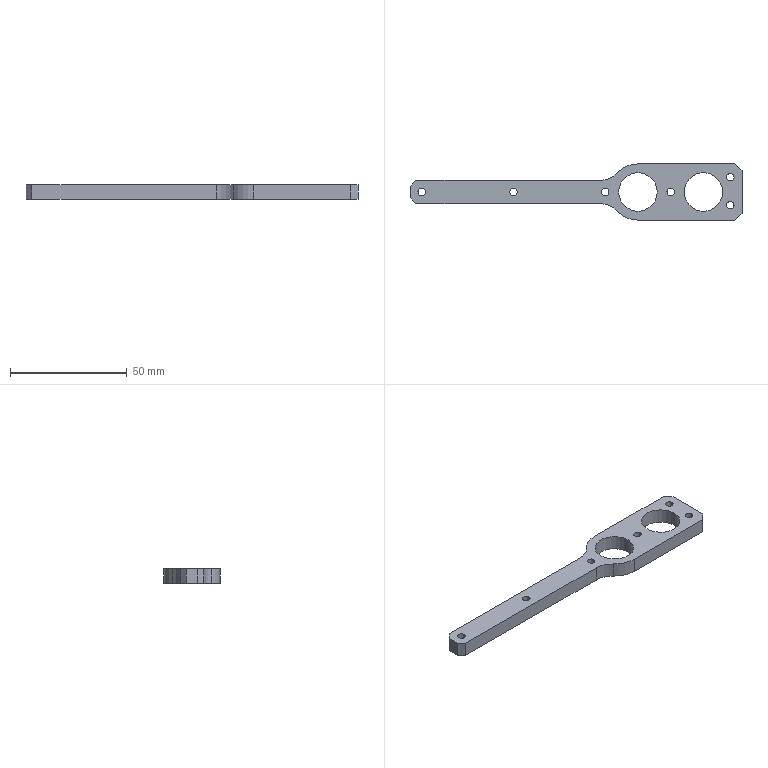Part | SolidWorks | features BaseBody 1 | 1 solid | 32 faces | box 142 x 24 x 6.35 mm | volume 10590 mm3 | cylinder 20 | plane 12 | commonest cylinder face diameters 3.2 x12 16.51 x4 20 x2 24 x2
STEP:
#1=CARTESIAN_POINT('',(-37.329,0.,6.35));
#2=VERTEX_POINT('',#1);
#3=CARTESIAN_POINT('',(-34.129,0.,6.35));
#4=VERTEX_POINT('',#3);
#5=CARTESIAN_POINT('',(-35.729,0.,6.35));
#6=DIRECTION('',(0.,0.,1.));
#7=DIRECTION('',(-1.,0.,0.));
#8=AXIS2_PLACEMENT_3D('',#5,#6,#7);
#9=CIRCLE('',#8,1.6);
#10=EDGE_CURVE('',#2,#4,#9,.T.);
#11=ORIENTED_EDGE('',*,*,#10,.T.);
#12=CARTESIAN_POINT('',(-34.129,0.,0.));
#13=VERTEX_POINT('',#12);
#14=CARTESIAN_POINT('',(-34.129,0.,6.35));
#15=DIRECTION('',(0.,0.,-1.));
#16=VECTOR('',#15,1000.);
#17=LINE('',#14,#16);
#18=EDGE_CURVE('',#4,#13,#17,.T.);
#19=ORIENTED_EDGE('',*,*,#18,.T.);
#20=CARTESIAN_POINT('',(-37.329,0.,0.));
#21=VERTEX_POINT('',#20);
#22=CARTESIAN_POINT('',(-35.729,0.,0.));
#23=DIRECTION('',(0.,0.,-1.));
#24=DIRECTION('',(-1.,0.,0.));
#25=AXIS2_PLACEMENT_3D('',#22,#23,#24);
#26=CIRCLE('',#25,1.6);
#27=EDGE_CURVE('',#13,#21,#26,.T.);
#28=ORIENTED_EDGE('',*,*,#27,.T.);
#29=CARTESIAN_POINT('',(-37.329,0.,6.35));
#30=DIRECTION('',(0.,0.,-1.));
#31=VECTOR('',#30,1000.);
#32=LINE('',#29,#31);
#33=EDGE_CURVE('',#2,#21,#32,.T.);
#34=ORIENTED_EDGE('',*,*,#33,.F.);
#35=EDGE_LOOP('',(#11,#19,#28,#34));
#36=FACE_OUTER_BOUND('',#35,.T.);
#37=CARTESIAN_POINT('',(-35.729,0.,6.35));
#38=DIRECTION('',(0.,0.,-1.));
#39=DIRECTION('',(-1.,0.,0.));
#40=AXIS2_PLACEMENT_3D('',#37,#38,#39);
#41=CYLINDRICAL_SURFACE('',#40,1.6);
#42=ADVANCED_FACE('',(#36),#41,.F.);
#43=CARTESIAN_POINT('',(58.621,-5.603,6.35));
#44=VERTEX_POINT('',#43);
#45=CARTESIAN_POINT('',(55.421,-5.603,6.35));
#46=VERTEX_POINT('',#45);
#47=CARTESIAN_POINT('',(57.021,-5.603,6.35));
#48=DIRECTION('',(0.,0.,-1.));
#49=DIRECTION('',(-1.,0.,0.));
#50=AXIS2_PLACEMENT_3D('',#47,#48,#49);
#51=CIRCLE('',#50,1.6);
#52=EDGE_CURVE('',#44,#46,#51,.T.);
#53=ORIENTED_EDGE('',*,*,#52,.F.);
#54=CARTESIAN_POINT('',(58.621,-5.603,0.));
#55=VERTEX_POINT('',#54);
#56=CARTESIAN_POINT('',(58.621,-5.603,6.35));
#57=DIRECTION('',(0.,0.,-1.));
#58=VECTOR('',#57,1000.);
#59=LINE('',#56,#58);
#60=EDGE_CURVE('',#44,#55,#59,.T.);
#61=ORIENTED_EDGE('',*,*,#60,.T.);
#62=CARTESIAN_POINT('',(55.421,-5.603,0.));
#63=VERTEX_POINT('',#62);
#64=CARTESIAN_POINT('',(57.021,-5.603,0.));
#65=DIRECTION('',(0.,0.,-1.));
#66=DIRECTION('',(-1.,0.,0.));
#67=AXIS2_PLACEMENT_3D('',#64,#65,#66);
#68=CIRCLE('',#67,1.6);
#69=EDGE_CURVE('',#55,#63,#68,.T.);
#70=ORIENTED_EDGE('',*,*,#69,.T.);
#71=CARTESIAN_POINT('',(55.421,-5.603,6.35));
#72=DIRECTION('',(0.,0.,-1.));
#73=VECTOR('',#72,1000.);
#74=LINE('',#71,#73);
#75=EDGE_CURVE('',#46,#63,#74,.T.);
#76=ORIENTED_EDGE('',*,*,#75,.F.);
#77=EDGE_LOOP('',(#53,#61,#70,#76));
#78=FACE_OUTER_BOUND('',#77,.T.);
#79=CARTESIAN_POINT('',(57.021,-5.603,6.35));
#80=DIRECTION('',(0.,0.,-1.));
#81=DIRECTION('',(-1.,0.,0.));
#82=AXIS2_PLACEMENT_3D('',#79,#80,#81);
#83=CYLINDRICAL_SURFACE('',#82,1.6);
#84=ADVANCED_FACE('',(#78),#83,.F.);
#85=CARTESIAN_POINT('',(-73.379,0.,6.35));
#86=VERTEX_POINT('',#85);
#87=CARTESIAN_POINT('',(-76.579,0.,6.35));
#88=VERTEX_POINT('',#87);
#89=CARTESIAN_POINT('',(-74.979,0.,6.35));
#90=DIRECTION('',(0.,0.,-1.));
#91=DIRECTION('',(-1.,0.,0.));
#92=AXIS2_PLACEMENT_3D('',#89,#90,#91);
#93=CIRCLE('',#92,1.6);
#94=EDGE_CURVE('',#86,#88,#93,.T.);
#95=ORIENTED_EDGE('',*,*,#94,.F.);
#96=CARTESIAN_POINT('',(-73.379,0.,0.));
#97=VERTEX_POINT('',#96);
#98=CARTESIAN_POINT('',(-73.379,0.,6.35));
#99=DIRECTION('',(0.,0.,-1.));
#100=VECTOR('',#99,1000.);
#101=LINE('',#98,#100);
#102=EDGE_CURVE('',#86,#97,#101,.T.);
#103=ORIENTED_EDGE('',*,*,#102,.T.);
#104=CARTESIAN_POINT('',(-76.579,0.,0.));
#105=VERTEX_POINT('',#104);
#106=CARTESIAN_POINT('',(-74.979,0.,0.));
#107=DIRECTION('',(0.,0.,-1.));
#108=DIRECTION('',(-1.,0.,0.));
#109=AXIS2_PLACEMENT_3D('',#106,#107,#108);
#110=CIRCLE('',#109,1.6);
#111=EDGE_CURVE('',#97,#105,#110,.T.);
#112=ORIENTED_EDGE('',*,*,#111,.T.);
#113=CARTESIAN_POINT('',(-76.579,0.,6.35));
#114=DIRECTION('',(0.,0.,-1.));
#115=VECTOR('',#114,1000.);
#116=LINE('',#113,#115);
#117=EDGE_CURVE('',#88,#105,#116,.T.);
#118=ORIENTED_EDGE('',*,*,#117,.F.);
#119=EDGE_LOOP('',(#95,#103,#112,#118));
#120=FACE_OUTER_BOUND('',#119,.T.);
#121=CARTESIAN_POINT('',(-74.979,0.,6.35));
#122=DIRECTION('',(0.,0.,-1.));
#123=DIRECTION('',(-1.,0.,0.));
#124=AXIS2_PLACEMENT_3D('',#121,#122,#123);
#125=CYLINDRICAL_SURFACE('',#124,1.6);
#126=ADVANCED_FACE('',(#120),#125,.F.);
#127=CARTESIAN_POINT('',(33.121,0.,6.35));
#128=VERTEX_POINT('',#127);
#129=CARTESIAN_POINT('',(29.921,0.,6.35));
#130=VERTEX_POINT('',#129);
#131=CARTESIAN_POINT('',(31.521,0.,6.35));
#132=DIRECTION('',(0.,0.,-1.));
#133=DIRECTION('',(-1.,0.,0.));
#134=AXIS2_PLACEMENT_3D('',#131,#132,#133);
#135=CIRCLE('',#134,1.6);
#136=EDGE_CURVE('',#128,#130,#135,.T.);
#137=ORIENTED_EDGE('',*,*,#136,.F.);
#138=CARTESIAN_POINT('',(33.121,0.,0.));
#139=VERTEX_POINT('',#138);
#140=CARTESIAN_POINT('',(33.121,0.,6.35));
#141=DIRECTION('',(0.,0.,-1.));
#142=VECTOR('',#141,1000.);
#143=LINE('',#140,#142);
#144=EDGE_CURVE('',#128,#139,#143,.T.);
#145=ORIENTED_EDGE('',*,*,#144,.T.);
#146=CARTESIAN_POINT('',(29.921,0.,0.));
#147=VERTEX_POINT('',#146);
#148=CARTESIAN_POINT('',(31.521,0.,0.));
#149=DIRECTION('',(0.,0.,-1.));
#150=DIRECTION('',(-1.,0.,0.));
#151=AXIS2_PLACEMENT_3D('',#148,#149,#150);
#152=CIRCLE('',#151,1.6);
#153=EDGE_CURVE('',#139,#147,#152,.T.);
#154=ORIENTED_EDGE('',*,*,#153,.T.);
#155=CARTESIAN_POINT('',(29.921,0.,6.35));
#156=DIRECTION('',(0.,0.,-1.));
#157=VECTOR('',#156,1000.);
#158=LINE('',#155,#157);
#159=EDGE_CURVE('',#130,#147,#158,.T.);
#160=ORIENTED_EDGE('',*,*,#159,.F.);
#161=EDGE_LOOP('',(#137,#145,#154,#160));
#162=FACE_OUTER_BOUND('',#161,.T.);
#163=CARTESIAN_POINT('',(31.521,0.,6.35));
#164=DIRECTION('',(0.,0.,-1.));
#165=DIRECTION('',(-1.,0.,0.));
#166=AXIS2_PLACEMENT_3D('',#163,#164,#165);
#167=CYLINDRICAL_SURFACE('',#166,1.6);
#168=ADVANCED_FACE('',(#162),#167,.F.);
#169=CARTESIAN_POINT('',(25.776,0.,6.35));
#170=VERTEX_POINT('',#169);
#171=CARTESIAN_POINT('',(9.266,0.,6.35));
#172=VERTEX_POINT('',#171);
#173=CARTESIAN_POINT('',(17.521,0.,6.35));
#174=DIRECTION('',(0.,0.,-1.));
#175=DIRECTION('',(-1.,0.,0.));
#176=AXIS2_PLACEMENT_3D('',#173,#174,#175);
#177=CIRCLE('',#176,8.255);
#178=EDGE_CURVE('',#170,#172,#177,.T.);
#179=ORIENTED_EDGE('',*,*,#178,.F.);
#180=CARTESIAN_POINT('',(25.776,0.,0.));
#181=VERTEX_POINT('',#180);
#182=CARTESIAN_POINT('',(25.776,0.,6.35));
#183=DIRECTION('',(0.,0.,-1.));
#184=VECTOR('',#183,1000.);
#185=LINE('',#182,#184);
#186=EDGE_CURVE('',#170,#181,#185,.T.);
#187=ORIENTED_EDGE('',*,*,#186,.T.);
#188=CARTESIAN_POINT('',(9.266,0.,0.));
#189=VERTEX_POINT('',#188);
#190=CARTESIAN_POINT('',(17.521,0.,0.));
#191=DIRECTION('',(0.,0.,-1.));
#192=DIRECTION('',(-1.,0.,0.));
#193=AXIS2_PLACEMENT_3D('',#190,#191,#192);
#194=CIRCLE('',#193,8.255);
#195=EDGE_CURVE('',#181,#189,#194,.T.);
#196=ORIENTED_EDGE('',*,*,#195,.T.);
#197=CARTESIAN_POINT('',(9.266,0.,6.35));
#198=DIRECTION('',(0.,0.,-1.));
#199=VECTOR('',#198,1000.);
#200=LINE('',#197,#199);
#201=EDGE_CURVE('',#172,#189,#200,.T.);
#202=ORIENTED_EDGE('',*,*,#201,.F.);
#203=EDGE_LOOP('',(#179,#187,#196,#202));
#204=FACE_OUTER_BOUND('',#203,.T.);
#205=CARTESIAN_POINT('',(17.521,0.,6.35));
#206=DIRECTION('',(0.,0.,-1.));
#207=DIRECTION('',(-1.,0.,0.));
#208=AXIS2_PLACEMENT_3D('',#205,#206,#207);
#209=CYLINDRICAL_SURFACE('',#208,8.255);
#210=ADVANCED_FACE('',(#204),#209,.F.);
#211=CARTESIAN_POINT('',(5.121,0.,6.35));
#212=VERTEX_POINT('',#211);
#213=CARTESIAN_POINT('',(1.921,0.,6.35));
#214=VERTEX_POINT('',#213);
#215=CARTESIAN_POINT('',(3.521,0.,6.35));
#216=DIRECTION('',(0.,0.,-1.));
#217=DIRECTION('',(-1.,0.,0.));
#218=AXIS2_PLACEMENT_3D('',#215,#216,#217);
#219=CIRCLE('',#218,1.6);
#220=EDGE_CURVE('',#212,#214,#219,.T.);
#221=ORIENTED_EDGE('',*,*,#220,.F.);
#222=CARTESIAN_POINT('',(5.121,0.,0.));
#223=VERTEX_POINT('',#222);
#224=CARTESIAN_POINT('',(5.121,0.,6.35));
#225=DIRECTION('',(0.,0.,-1.));
#226=VECTOR('',#225,1000.);
#227=LINE('',#224,#226);
#228=EDGE_CURVE('',#212,#223,#227,.T.);
#229=ORIENTED_EDGE('',*,*,#228,.T.);
#230=CARTESIAN_POINT('',(1.921,0.,0.));
#231=VERTEX_POINT('',#230);
#232=CARTESIAN_POINT('',(3.521,0.,0.));
#233=DIRECTION('',(0.,0.,-1.));
#234=DIRECTION('',(-1.,0.,0.));
#235=AXIS2_PLACEMENT_3D('',#232,#233,#234);
#236=CIRCLE('',#235,1.6);
#237=EDGE_CURVE('',#223,#231,#236,.T.);
#238=ORIENTED_EDGE('',*,*,#237,.T.);
#239=CARTESIAN_POINT('',(1.921,0.,6.35));
#240=DIRECTION('',(0.,0.,-1.));
#241=VECTOR('',#240,1000.);
#242=LINE('',#239,#241);
#243=EDGE_CURVE('',#214,#231,#242,.T.);
#244=ORIENTED_EDGE('',*,*,#243,.F.);
#245=EDGE_LOOP('',(#221,#229,#238,#244));
#246=FACE_OUTER_BOUND('',#245,.T.);
#247=CARTESIAN_POINT('',(3.521,0.,6.35));
#248=DIRECTION('',(0.,0.,-1.));
#249=DIRECTION('',(-1.,0.,0.));
#250=AXIS2_PLACEMENT_3D('',#247,#248,#249);
#251=CYLINDRICAL_SURFACE('',#250,1.6);
#252=ADVANCED_FACE('',(#246),#251,.F.);
#253=CARTESIAN_POINT('',(58.621,6.302,6.35));
#254=VERTEX_POINT('',#253);
#255=CARTESIAN_POINT('',(55.421,6.302,6.35));
#256=VERTEX_POINT('',#255);
#257=CARTESIAN_POINT('',(57.021,6.302,6.35));
#258=DIRECTION('',(0.,0.,-1.));
#259=DIRECTION('',(-1.,0.,0.));
#260=AXIS2_PLACEMENT_3D('',#257,#258,#259);
#261=CIRCLE('',#260,1.6);
#262=EDGE_CURVE('',#254,#256,#261,.T.);
#263=ORIENTED_EDGE('',*,*,#262,.F.);
#264=CARTESIAN_POINT('',(58.621,6.302,0.));
#265=VERTEX_POINT('',#264);
#266=CARTESIAN_POINT('',(58.621,6.302,6.35));
#267=DIRECTION('',(0.,0.,-1.));
#268=VECTOR('',#267,1000.);
#269=LINE('',#266,#268);
#270=EDGE_CURVE('',#254,#265,#269,.T.);
#271=ORIENTED_EDGE('',*,*,#270,.T.);
#272=CARTESIAN_POINT('',(55.421,6.302,0.));
#273=VERTEX_POINT('',#272);
#274=CARTESIAN_POINT('',(57.021,6.302,0.));
#275=DIRECTION('',(0.,0.,-1.));
#276=DIRECTION('',(-1.,0.,0.));
#277=AXIS2_PLACEMENT_3D('',#274,#275,#276);
#278=CIRCLE('',#277,1.6);
#279=EDGE_CURVE('',#265,#273,#278,.T.);
#280=ORIENTED_EDGE('',*,*,#279,.T.);
#281=CARTESIAN_POINT('',(55.421,6.302,6.35));
#282=DIRECTION('',(0.,0.,-1.));
#283=VECTOR('',#282,1000.);
#284=LINE('',#281,#283);
#285=EDGE_CURVE('',#256,#273,#284,.T.);
#286=ORIENTED_EDGE('',*,*,#285,.F.);
#287=EDGE_LOOP('',(#263,#271,#280,#286));
#288=FACE_OUTER_BOUND('',#287,.T.);
#289=CARTESIAN_POINT('',(57.021,6.302,6.35));
#290=DIRECTION('',(0.,0.,-1.));
#291=DIRECTION('',(-1.,0.,0.));
#292=AXIS2_PLACEMENT_3D('',#289,#290,#291);
#293=CYLINDRICAL_SURFACE('',#292,1.6);
#294=ADVANCED_FACE('',(#288),#293,.F.);
#295=CARTESIAN_POINT('',(53.776,0.,6.35));
#296=VERTEX_POINT('',#295);
#297=CARTESIAN_POINT('',(37.266,0.,6.35));
#298=VERTEX_POINT('',#297);
#299=CARTESIAN_POINT('',(45.521,0.,6.35));
#300=DIRECTION('',(0.,0.,-1.));
#301=DIRECTION('',(-1.,0.,0.));
#302=AXIS2_PLACEMENT_3D('',#299,#300,#301);
#303=CIRCLE('',#302,8.255);
#304=EDGE_CURVE('',#296,#298,#303,.T.);
#305=ORIENTED_EDGE('',*,*,#304,.F.);
#306=CARTESIAN_POINT('',(53.776,0.,0.));
#307=VERTEX_POINT('',#306);
#308=CARTESIAN_POINT('',(53.776,0.,6.35));
#309=DIRECTION('',(0.,0.,-1.));
#310=VECTOR('',#309,1000.);
#311=LINE('',#308,#310);
#312=EDGE_CURVE('',#296,#307,#311,.T.);
#313=ORIENTED_EDGE('',*,*,#312,.T.);
#314=CARTESIAN_POINT('',(37.266,0.,0.));
#315=VERTEX_POINT('',#314);
#316=CARTESIAN_POINT('',(45.521,0.,0.));
#317=DIRECTION('',(0.,0.,-1.));
#318=DIRECTION('',(-1.,0.,0.));
#319=AXIS2_PLACEMENT_3D('',#316,#317,#318);
#320=CIRCLE('',#319,8.255);
#321=EDGE_CURVE('',#307,#315,#320,.T.);
#322=ORIENTED_EDGE('',*,*,#321,.T.);
#323=CARTESIAN_POINT('',(37.266,0.,6.35));
#324=DIRECTION('',(0.,0.,-1.));
#325=VECTOR('',#324,1000.);
#326=LINE('',#323,#325);
#327=EDGE_CURVE('',#298,#315,#326,.T.);
#328=ORIENTED_EDGE('',*,*,#327,.F.);
#329=EDGE_LOOP('',(#305,#313,#322,#328));
#330=FACE_OUTER_BOUND('',#329,.T.);
#331=CARTESIAN_POINT('',(45.521,0.,6.35));
#332=DIRECTION('',(0.,0.,-1.));
#333=DIRECTION('',(-1.,0.,0.));
#334=AXIS2_PLACEMENT_3D('',#331,#332,#333);
#335=CYLINDRICAL_SURFACE('',#334,8.255);
#336=ADVANCED_FACE('',(#330),#335,.F.);
#337=ORIENTED_EDGE('',*,*,#18,.F.);
#338=CARTESIAN_POINT('',(-35.729,0.,6.35));
#339=DIRECTION('',(0.,0.,1.));
#340=DIRECTION('',(-1.,0.,0.));
#341=AXIS2_PLACEMENT_3D('',#338,#339,#340);
#342=CIRCLE('',#341,1.6);
#343=EDGE_CURVE('',#4,#2,#342,.T.);
#344=ORIENTED_EDGE('',*,*,#343,.T.);
#345=ORIENTED_EDGE('',*,*,#33,.T.);
#346=CARTESIAN_POINT('',(-35.729,0.,0.));
#347=DIRECTION('',(0.,0.,-1.));
#348=DIRECTION('',(-1.,0.,0.));
#349=AXIS2_PLACEMENT_3D('',#346,#347,#348);
#350=CIRCLE('',#349,1.6);
#351=EDGE_CURVE('',#21,#13,#350,.T.);
#352=ORIENTED_EDGE('',*,*,#351,.T.);
#353=EDGE_LOOP('',(#337,#344,#345,#352));
#354=FACE_OUTER_BOUND('',#353,.T.);
#355=CARTESIAN_POINT('',(-35.729,0.,6.35));
#356=DIRECTION('',(0.,0.,-1.));
#357=DIRECTION('',(-1.,0.,0.));
#358=AXIS2_PLACEMENT_3D('',#355,#356,#357);
#359=CYLINDRICAL_SURFACE('',#358,1.6);
#360=ADVANCED_FACE('',(#354),#359,.F.);
#361=ORIENTED_EDGE('',*,*,#351,.F.);
#362=ORIENTED_EDGE('',*,*,#27,.F.);
#363=EDGE_LOOP('',(#361,#362));
#364=FACE_BOUND('',#363,.T.);
#365=CARTESIAN_POINT('',(57.021,-5.603,0.));
#366=DIRECTION('',(0.,0.,-1.));
#367=DIRECTION('',(-1.,0.,0.));
#368=AXIS2_PLACEMENT_3D('',#365,#366,#367);
#369=CIRCLE('',#368,1.6);
#370=EDGE_CURVE('',#63,#55,#369,.T.);
#371=ORIENTED_EDGE('',*,*,#370,.F.);
#372=ORIENTED_EDGE('',*,*,#69,.F.);
#373=EDGE_LOOP('',(#371,#372));
#374=FACE_BOUND('',#373,.T.);
#375=CARTESIAN_POINT('',(-74.979,0.,0.));
#376=DIRECTION('',(0.,0.,-1.));
#377=DIRECTION('',(-1.,0.,0.));
#378=AXIS2_PLACEMENT_3D('',#375,#376,#377);
#379=CIRCLE('',#378,1.6);
#380=EDGE_CURVE('',#105,#97,#379,.T.);
#381=ORIENTED_EDGE('',*,*,#380,.F.);
#382=ORIENTED_EDGE('',*,*,#111,.F.);
#383=EDGE_LOOP('',(#381,#382));
#384=FACE_BOUND('',#383,.T.);
#385=CARTESIAN_POINT('',(31.521,0.,0.));
#386=DIRECTION('',(0.,0.,-1.));
#387=DIRECTION('',(-1.,0.,0.));
#388=AXIS2_PLACEMENT_3D('',#385,#386,#387);
#389=CIRCLE('',#388,1.6);
#390=EDGE_CURVE('',#147,#139,#389,.T.);
#391=ORIENTED_EDGE('',*,*,#390,.F.);
#392=ORIENTED_EDGE('',*,*,#153,.F.);
#393=EDGE_LOOP('',(#391,#392));
#394=FACE_BOUND('',#393,.T.);
#395=CARTESIAN_POINT('',(17.521,0.,0.));
#396=DIRECTION('',(0.,0.,-1.));
#397=DIRECTION('',(-1.,0.,0.));
#398=AXIS2_PLACEMENT_3D('',#395,#396,#397);
#399=CIRCLE('',#398,8.255);
#400=EDGE_CURVE('',#189,#181,#399,.T.);
#401=ORIENTED_EDGE('',*,*,#400,.F.);
#402=ORIENTED_EDGE('',*,*,#195,.F.);
#403=EDGE_LOOP('',(#401,#402));
#404=FACE_BOUND('',#403,.T.);
#405=CARTESIAN_POINT('',(3.521,0.,0.));
#406=DIRECTION('',(0.,0.,-1.));
#407=DIRECTION('',(-1.,0.,0.));
#408=AXIS2_PLACEMENT_3D('',#405,#406,#407);
#409=CIRCLE('',#408,1.6);
#410=EDGE_CURVE('',#231,#223,#409,.T.);
#411=ORIENTED_EDGE('',*,*,#410,.F.);
#412=ORIENTED_EDGE('',*,*,#237,.F.);
#413=EDGE_LOOP('',(#411,#412));
#414=FACE_BOUND('',#413,.T.);
#415=CARTESIAN_POINT('',(57.021,6.302,0.));
#416=DIRECTION('',(0.,0.,-1.));
#417=DIRECTION('',(-1.,0.,0.));
#418=AXIS2_PLACEMENT_3D('',#415,#416,#417);
#419=CIRCLE('',#418,1.6);
#420=EDGE_CURVE('',#273,#265,#419,.T.);
#421=ORIENTED_EDGE('',*,*,#420,.F.);
#422=ORIENTED_EDGE('',*,*,#279,.F.);
#423=EDGE_LOOP('',(#421,#422));
#424=FACE_BOUND('',#423,.T.);
#425=CARTESIAN_POINT('',(45.521,0.,0.));
#426=DIRECTION('',(0.,0.,-1.));
#427=DIRECTION('',(-1.,0.,0.));
#428=AXIS2_PLACEMENT_3D('',#425,#426,#427);
#429=CIRCLE('',#428,8.255);
#430=EDGE_CURVE('',#315,#307,#429,.T.);
#431=ORIENTED_EDGE('',*,*,#430,.F.);
#432=ORIENTED_EDGE('',*,*,#321,.F.);
#433=EDGE_LOOP('',(#431,#432));
#434=FACE_BOUND('',#433,.T.);
#435=CARTESIAN_POINT('',(8.742,8.182,0.));
#436=VERTEX_POINT('',#435);
#437=CARTESIAN_POINT('',(1.427,5.,0.));
#438=VERTEX_POINT('',#437);
#439=CARTESIAN_POINT('',(1.427,15.,0.));
#440=DIRECTION('',(0.,0.,-1.));
#441=DIRECTION('',(-1.,0.,0.));
#442=AXIS2_PLACEMENT_3D('',#439,#440,#441);
#443=CIRCLE('',#442,10.);
#444=EDGE_CURVE('',#436,#438,#443,.T.);
#445=ORIENTED_EDGE('',*,*,#444,.F.);
#446=CARTESIAN_POINT('',(17.521,12.,0.));
#447=VERTEX_POINT('',#446);
#448=CARTESIAN_POINT('',(17.521,0.,0.));
#449=DIRECTION('',(0.,0.,1.));
#450=DIRECTION('',(-1.,0.,0.));
#451=AXIS2_PLACEMENT_3D('',#448,#449,#450);
#452=CIRCLE('',#451,12.);
#453=EDGE_CURVE('',#447,#436,#452,.T.);
#454=ORIENTED_EDGE('',*,*,#453,.F.);
#455=CARTESIAN_POINT('',(59.021,12.,0.));
#456=VERTEX_POINT('',#455);
#457=CARTESIAN_POINT('',(-8.979,12.,0.));
#458=DIRECTION('',(-1.,0.,0.));
#459=VECTOR('',#458,1000.);
#460=LINE('',#457,#459);
#461=EDGE_CURVE('',#456,#447,#460,.T.);
#462=ORIENTED_EDGE('',*,*,#461,.F.);
#463=CARTESIAN_POINT('',(62.021,9.,0.));
#464=VERTEX_POINT('',#463);
#465=CARTESIAN_POINT('',(59.021,12.,0.));
#466=DIRECTION('',(-0.7071,0.7071,0.));
#467=VECTOR('',#466,1000.);
#468=LINE('',#465,#467);
#469=EDGE_CURVE('',#464,#456,#468,.T.);
#470=ORIENTED_EDGE('',*,*,#469,.F.);
#471=CARTESIAN_POINT('',(62.021,-9.,0.));
#472=VERTEX_POINT('',#471);
#473=CARTESIAN_POINT('',(62.021,0.,0.));
#474=DIRECTION('',(0.,1.,0.));
#475=VECTOR('',#474,1000.);
#476=LINE('',#473,#475);
#477=EDGE_CURVE('',#472,#464,#476,.T.);
#478=ORIENTED_EDGE('',*,*,#477,.F.);
#479=CARTESIAN_POINT('',(59.021,-12.,0.));
#480=VERTEX_POINT('',#479);
#481=CARTESIAN_POINT('',(62.021,-9.,0.));
#482=DIRECTION('',(0.7071,0.7071,0.));
#483=VECTOR('',#482,1000.);
#484=LINE('',#481,#483);
#485=EDGE_CURVE('',#480,#472,#484,.T.);
#486=ORIENTED_EDGE('',*,*,#485,.F.);
#487=CARTESIAN_POINT('',(17.521,-12.,0.));
#488=VERTEX_POINT('',#487);
#489=CARTESIAN_POINT('',(-8.979,-12.,0.));
#490=DIRECTION('',(1.,0.,0.));
#491=VECTOR('',#490,1000.);
#492=LINE('',#489,#491);
#493=EDGE_CURVE('',#488,#480,#492,.T.);
#494=ORIENTED_EDGE('',*,*,#493,.F.);
#495=CARTESIAN_POINT('',(8.742,-8.182,0.));
#496=VERTEX_POINT('',#495);
#497=CARTESIAN_POINT('',(17.521,0.,0.));
#498=DIRECTION('',(0.,0.,1.));
#499=DIRECTION('',(-1.,0.,0.));
#500=AXIS2_PLACEMENT_3D('',#497,#498,#499);
#501=CIRCLE('',#500,12.);
#502=EDGE_CURVE('',#496,#488,#501,.T.);
#503=ORIENTED_EDGE('',*,*,#502,.F.);
#504=CARTESIAN_POINT('',(1.427,-5.,0.));
#505=VERTEX_POINT('',#504);
#506=CARTESIAN_POINT('',(1.427,-15.,0.));
#507=DIRECTION('',(0.,0.,-1.));
#508=DIRECTION('',(-1.,0.,0.));
#509=AXIS2_PLACEMENT_3D('',#506,#507,#508);
#510=CIRCLE('',#509,10.);
#511=EDGE_CURVE('',#505,#496,#510,.T.);
#512=ORIENTED_EDGE('',*,*,#511,.F.);
#513=CARTESIAN_POINT('',(-77.439,-5.,0.));
#514=VERTEX_POINT('',#513);
#515=CARTESIAN_POINT('',(-8.979,-5.,0.));
#516=DIRECTION('',(1.,0.,0.));
#517=VECTOR('',#516,1000.);
#518=LINE('',#515,#517);
#519=EDGE_CURVE('',#514,#505,#518,.T.);
#520=ORIENTED_EDGE('',*,*,#519,.F.);
#521=CARTESIAN_POINT('',(-79.979,-2.46,0.));
#522=VERTEX_POINT('',#521);
#523=CARTESIAN_POINT('',(-77.439,-5.,0.));
#524=DIRECTION('',(0.7071,-0.7071,0.));
#525=VECTOR('',#524,1000.);
#526=LINE('',#523,#525);
#527=EDGE_CURVE('',#522,#514,#526,.T.);
#528=ORIENTED_EDGE('',*,*,#527,.F.);
#529=CARTESIAN_POINT('',(-79.979,2.46,0.));
#530=VERTEX_POINT('',#529);
#531=CARTESIAN_POINT('',(-79.979,0.,0.));
#532=DIRECTION('',(0.,-1.,0.));
#533=VECTOR('',#532,1000.);
#534=LINE('',#531,#533);
#535=EDGE_CURVE('',#530,#522,#534,.T.);
#536=ORIENTED_EDGE('',*,*,#535,.F.);
#537=CARTESIAN_POINT('',(-77.439,5.,0.));
#538=VERTEX_POINT('',#537);
#539=CARTESIAN_POINT('',(-79.979,2.46,0.));
#540=DIRECTION('',(-0.7071,-0.7071,0.));
#541=VECTOR('',#540,1000.);
#542=LINE('',#539,#541);
#543=EDGE_CURVE('',#538,#530,#542,.T.);
#544=ORIENTED_EDGE('',*,*,#543,.F.);
#545=CARTESIAN_POINT('',(-8.979,5.,0.));
#546=DIRECTION('',(-1.,0.,0.));
#547=VECTOR('',#546,1000.);
#548=LINE('',#545,#547);
#549=EDGE_CURVE('',#438,#538,#548,.T.);
#550=ORIENTED_EDGE('',*,*,#549,.F.);
#551=EDGE_LOOP('',(#445,#454,#462,#470,#478,#486,#494,#503,#512,#520,#528,#536,#544,#550));
#552=FACE_OUTER_BOUND('',#551,.T.);
#553=CARTESIAN_POINT('',(-79.979,-12.,0.));
#554=DIRECTION('',(0.,0.,1.));
#555=DIRECTION('',(1.,0.,0.));
#556=AXIS2_PLACEMENT_3D('',#553,#554,#555);
#557=PLANE('',#556);
#558=ADVANCED_FACE('',(#364,#374,#384,#394,#404,#414,#424,#434,#552),#557,.F.);
#559=ORIENTED_EDGE('',*,*,#10,.F.);
#560=ORIENTED_EDGE('',*,*,#343,.F.);
#561=EDGE_LOOP('',(#559,#560));
#562=FACE_BOUND('',#561,.T.);
#563=CARTESIAN_POINT('',(57.021,-5.603,6.35));
#564=DIRECTION('',(0.,0.,-1.));
#565=DIRECTION('',(-1.,0.,0.));
#566=AXIS2_PLACEMENT_3D('',#563,#564,#565);
#567=CIRCLE('',#566,1.6);
#568=EDGE_CURVE('',#46,#44,#567,.T.);
#569=ORIENTED_EDGE('',*,*,#568,.T.);
#570=ORIENTED_EDGE('',*,*,#52,.T.);
#571=EDGE_LOOP('',(#569,#570));
#572=FACE_BOUND('',#571,.T.);
#573=CARTESIAN_POINT('',(-74.979,0.,6.35));
#574=DIRECTION('',(0.,0.,-1.));
#575=DIRECTION('',(-1.,0.,0.));
#576=AXIS2_PLACEMENT_3D('',#573,#574,#575);
#577=CIRCLE('',#576,1.6);
#578=EDGE_CURVE('',#88,#86,#577,.T.);
#579=ORIENTED_EDGE('',*,*,#578,.T.);
#580=ORIENTED_EDGE('',*,*,#94,.T.);
#581=EDGE_LOOP('',(#579,#580));
#582=FACE_BOUND('',#581,.T.);
#583=CARTESIAN_POINT('',(31.521,0.,6.35));
#584=DIRECTION('',(0.,0.,-1.));
#585=DIRECTION('',(-1.,0.,0.));
#586=AXIS2_PLACEMENT_3D('',#583,#584,#585);
#587=CIRCLE('',#586,1.6);
#588=EDGE_CURVE('',#130,#128,#587,.T.);
#589=ORIENTED_EDGE('',*,*,#588,.T.);
#590=ORIENTED_EDGE('',*,*,#136,.T.);
#591=EDGE_LOOP('',(#589,#590));
#592=FACE_BOUND('',#591,.T.);
#593=CARTESIAN_POINT('',(17.521,0.,6.35));
#594=DIRECTION('',(0.,0.,-1.));
#595=DIRECTION('',(-1.,0.,0.));
#596=AXIS2_PLACEMENT_3D('',#593,#594,#595);
#597=CIRCLE('',#596,8.255);
#598=EDGE_CURVE('',#172,#170,#597,.T.);
#599=ORIENTED_EDGE('',*,*,#598,.T.);
#600=ORIENTED_EDGE('',*,*,#178,.T.);
#601=EDGE_LOOP('',(#599,#600));
#602=FACE_BOUND('',#601,.T.);
#603=CARTESIAN_POINT('',(3.521,0.,6.35));
#604=DIRECTION('',(0.,0.,-1.));
#605=DIRECTION('',(-1.,0.,0.));
#606=AXIS2_PLACEMENT_3D('',#603,#604,#605);
#607=CIRCLE('',#606,1.6);
#608=EDGE_CURVE('',#214,#212,#607,.T.);
#609=ORIENTED_EDGE('',*,*,#608,.T.);
#610=ORIENTED_EDGE('',*,*,#220,.T.);
#611=EDGE_LOOP('',(#609,#610));
#612=FACE_BOUND('',#611,.T.);
#613=CARTESIAN_POINT('',(57.021,6.302,6.35));
#614=DIRECTION('',(0.,0.,-1.));
#615=DIRECTION('',(-1.,0.,0.));
#616=AXIS2_PLACEMENT_3D('',#613,#614,#615);
#617=CIRCLE('',#616,1.6);
#618=EDGE_CURVE('',#256,#254,#617,.T.);
#619=ORIENTED_EDGE('',*,*,#618,.T.);
#620=ORIENTED_EDGE('',*,*,#262,.T.);
#621=EDGE_LOOP('',(#619,#620));
#622=FACE_BOUND('',#621,.T.);
#623=CARTESIAN_POINT('',(45.521,0.,6.35));
#624=DIRECTION('',(0.,0.,-1.));
#625=DIRECTION('',(-1.,0.,0.));
#626=AXIS2_PLACEMENT_3D('',#623,#624,#625);
#627=CIRCLE('',#626,8.255);
#628=EDGE_CURVE('',#298,#296,#627,.T.);
#629=ORIENTED_EDGE('',*,*,#628,.T.);
#630=ORIENTED_EDGE('',*,*,#304,.T.);
#631=EDGE_LOOP('',(#629,#630));
#632=FACE_BOUND('',#631,.T.);
#633=CARTESIAN_POINT('',(17.521,12.,6.35));
#634=VERTEX_POINT('',#633);
#635=CARTESIAN_POINT('',(8.742,8.182,6.35));
#636=VERTEX_POINT('',#635);
#637=CARTESIAN_POINT('',(17.521,0.,6.35));
#638=DIRECTION('',(0.,0.,1.));
#639=DIRECTION('',(-1.,0.,0.));
#640=AXIS2_PLACEMENT_3D('',#637,#638,#639);
#641=CIRCLE('',#640,12.);
#642=EDGE_CURVE('',#634,#636,#641,.T.);
#643=ORIENTED_EDGE('',*,*,#642,.T.);
#644=CARTESIAN_POINT('',(1.427,5.,6.35));
#645=VERTEX_POINT('',#644);
#646=CARTESIAN_POINT('',(1.427,15.,6.35));
#647=DIRECTION('',(0.,0.,-1.));
#648=DIRECTION('',(-1.,0.,0.));
#649=AXIS2_PLACEMENT_3D('',#646,#647,#648);
#650=CIRCLE('',#649,10.);
#651=EDGE_CURVE('',#636,#645,#650,.T.);
#652=ORIENTED_EDGE('',*,*,#651,.T.);
#653=CARTESIAN_POINT('',(-77.439,5.,6.35));
#654=VERTEX_POINT('',#653);
#655=CARTESIAN_POINT('',(-8.979,5.,6.35));
#656=DIRECTION('',(-1.,0.,0.));
#657=VECTOR('',#656,1000.);
#658=LINE('',#655,#657);
#659=EDGE_CURVE('',#645,#654,#658,.T.);
#660=ORIENTED_EDGE('',*,*,#659,.T.);
#661=CARTESIAN_POINT('',(-79.979,2.46,6.35));
#662=VERTEX_POINT('',#661);
#663=CARTESIAN_POINT('',(-77.439,5.,6.35));
#664=DIRECTION('',(-0.7071,-0.7071,0.));
#665=VECTOR('',#664,1000.);
#666=LINE('',#663,#665);
#667=EDGE_CURVE('',#654,#662,#666,.T.);
#668=ORIENTED_EDGE('',*,*,#667,.T.);
#669=CARTESIAN_POINT('',(-79.979,-2.46,6.35));
#670=VERTEX_POINT('',#669);
#671=CARTESIAN_POINT('',(-79.979,0.,6.35));
#672=DIRECTION('',(0.,-1.,0.));
#673=VECTOR('',#672,1000.);
#674=LINE('',#671,#673);
#675=EDGE_CURVE('',#662,#670,#674,.T.);
#676=ORIENTED_EDGE('',*,*,#675,.T.);
#677=CARTESIAN_POINT('',(-77.439,-5.,6.35));
#678=VERTEX_POINT('',#677);
#679=CARTESIAN_POINT('',(-79.979,-2.46,6.35));
#680=DIRECTION('',(0.7071,-0.7071,0.));
#681=VECTOR('',#680,1000.);
#682=LINE('',#679,#681);
#683=EDGE_CURVE('',#670,#678,#682,.T.);
#684=ORIENTED_EDGE('',*,*,#683,.T.);
#685=CARTESIAN_POINT('',(1.427,-5.,6.35));
#686=VERTEX_POINT('',#685);
#687=CARTESIAN_POINT('',(-8.979,-5.,6.35));
#688=DIRECTION('',(1.,0.,0.));
#689=VECTOR('',#688,1000.);
#690=LINE('',#687,#689);
#691=EDGE_CURVE('',#678,#686,#690,.T.);
#692=ORIENTED_EDGE('',*,*,#691,.T.);
#693=CARTESIAN_POINT('',(8.742,-8.182,6.35));
#694=VERTEX_POINT('',#693);
#695=CARTESIAN_POINT('',(1.427,-15.,6.35));
#696=DIRECTION('',(0.,0.,-1.));
#697=DIRECTION('',(-1.,0.,0.));
#698=AXIS2_PLACEMENT_3D('',#695,#696,#697);
#699=CIRCLE('',#698,10.);
#700=EDGE_CURVE('',#686,#694,#699,.T.);
#701=ORIENTED_EDGE('',*,*,#700,.T.);
#702=CARTESIAN_POINT('',(17.521,-12.,6.35));
#703=VERTEX_POINT('',#702);
#704=CARTESIAN_POINT('',(17.521,0.,6.35));
#705=DIRECTION('',(0.,0.,1.));
#706=DIRECTION('',(-1.,0.,0.));
#707=AXIS2_PLACEMENT_3D('',#704,#705,#706);
#708=CIRCLE('',#707,12.);
#709=EDGE_CURVE('',#694,#703,#708,.T.);
#710=ORIENTED_EDGE('',*,*,#709,.T.);
#711=CARTESIAN_POINT('',(59.021,-12.,6.35));
#712=VERTEX_POINT('',#711);
#713=CARTESIAN_POINT('',(-8.979,-12.,6.35));
#714=DIRECTION('',(1.,0.,0.));
#715=VECTOR('',#714,1000.);
#716=LINE('',#713,#715);
#717=EDGE_CURVE('',#703,#712,#716,.T.);
#718=ORIENTED_EDGE('',*,*,#717,.T.);
#719=CARTESIAN_POINT('',(62.021,-9.,6.35));
#720=VERTEX_POINT('',#719);
#721=CARTESIAN_POINT('',(59.021,-12.,6.35));
#722=DIRECTION('',(0.7071,0.7071,0.));
#723=VECTOR('',#722,1000.);
#724=LINE('',#721,#723);
#725=EDGE_CURVE('',#712,#720,#724,.T.);
#726=ORIENTED_EDGE('',*,*,#725,.T.);
#727=CARTESIAN_POINT('',(62.021,9.,6.35));
#728=VERTEX_POINT('',#727);
#729=CARTESIAN_POINT('',(62.021,0.,6.35));
#730=DIRECTION('',(0.,1.,0.));
#731=VECTOR('',#730,1000.);
#732=LINE('',#729,#731);
#733=EDGE_CURVE('',#720,#728,#732,.T.);
#734=ORIENTED_EDGE('',*,*,#733,.T.);
#735=CARTESIAN_POINT('',(59.021,12.,6.35));
#736=VERTEX_POINT('',#735);
#737=CARTESIAN_POINT('',(62.021,9.,6.35));
#738=DIRECTION('',(-0.7071,0.7071,0.));
#739=VECTOR('',#738,1000.);
#740=LINE('',#737,#739);
#741=EDGE_CURVE('',#728,#736,#740,.T.);
#742=ORIENTED_EDGE('',*,*,#741,.T.);
#743=CARTESIAN_POINT('',(-8.979,12.,6.35));
#744=DIRECTION('',(-1.,0.,0.));
#745=VECTOR('',#744,1000.);
#746=LINE('',#743,#745);
#747=EDGE_CURVE('',#736,#634,#746,.T.);
#748=ORIENTED_EDGE('',*,*,#747,.T.);
#749=EDGE_LOOP('',(#643,#652,#660,#668,#676,#684,#692,#701,#710,#718,#726,#734,#742,#748));
#750=FACE_OUTER_BOUND('',#749,.T.);
#751=CARTESIAN_POINT('',(-79.979,-12.,6.35));
#752=DIRECTION('',(0.,0.,1.));
#753=DIRECTION('',(1.,0.,0.));
#754=AXIS2_PLACEMENT_3D('',#751,#752,#753);
#755=PLANE('',#754);
#756=ADVANCED_FACE('',(#562,#572,#582,#592,#602,#612,#622,#632,#750),#755,.T.);
#757=ORIENTED_EDGE('',*,*,#60,.F.);
#758=ORIENTED_EDGE('',*,*,#568,.F.);
#759=ORIENTED_EDGE('',*,*,#75,.T.);
#760=ORIENTED_EDGE('',*,*,#370,.T.);
#761=EDGE_LOOP('',(#757,#758,#759,#760));
#762=FACE_OUTER_BOUND('',#761,.T.);
#763=CARTESIAN_POINT('',(57.021,-5.603,6.35));
#764=DIRECTION('',(0.,0.,-1.));
#765=DIRECTION('',(-1.,0.,0.));
#766=AXIS2_PLACEMENT_3D('',#763,#764,#765);
#767=CYLINDRICAL_SURFACE('',#766,1.6);
#768=ADVANCED_FACE('',(#762),#767,.F.);
#769=ORIENTED_EDGE('',*,*,#102,.F.);
#770=ORIENTED_EDGE('',*,*,#578,.F.);
#771=ORIENTED_EDGE('',*,*,#117,.T.);
#772=ORIENTED_EDGE('',*,*,#380,.T.);
#773=EDGE_LOOP('',(#769,#770,#771,#772));
#774=FACE_OUTER_BOUND('',#773,.T.);
#775=CARTESIAN_POINT('',(-74.979,0.,6.35));
#776=DIRECTION('',(0.,0.,-1.));
#777=DIRECTION('',(-1.,0.,0.));
#778=AXIS2_PLACEMENT_3D('',#775,#776,#777);
#779=CYLINDRICAL_SURFACE('',#778,1.6);
#780=ADVANCED_FACE('',(#774),#779,.F.);
#781=ORIENTED_EDGE('',*,*,#144,.F.);
#782=ORIENTED_EDGE('',*,*,#588,.F.);
#783=ORIENTED_EDGE('',*,*,#159,.T.);
#784=ORIENTED_EDGE('',*,*,#390,.T.);
#785=EDGE_LOOP('',(#781,#782,#783,#784));
#786=FACE_OUTER_BOUND('',#785,.T.);
#787=CARTESIAN_POINT('',(31.521,0.,6.35));
#788=DIRECTION('',(0.,0.,-1.));
#789=DIRECTION('',(-1.,0.,0.));
#790=AXIS2_PLACEMENT_3D('',#787,#788,#789);
#791=CYLINDRICAL_SURFACE('',#790,1.6);
#792=ADVANCED_FACE('',(#786),#791,.F.);
#793=ORIENTED_EDGE('',*,*,#186,.F.);
#794=ORIENTED_EDGE('',*,*,#598,.F.);
#795=ORIENTED_EDGE('',*,*,#201,.T.);
#796=ORIENTED_EDGE('',*,*,#400,.T.);
#797=EDGE_LOOP('',(#793,#794,#795,#796));
#798=FACE_OUTER_BOUND('',#797,.T.);
#799=CARTESIAN_POINT('',(17.521,0.,6.35));
#800=DIRECTION('',(0.,0.,-1.));
#801=DIRECTION('',(-1.,0.,0.));
#802=AXIS2_PLACEMENT_3D('',#799,#800,#801);
#803=CYLINDRICAL_SURFACE('',#802,8.255);
#804=ADVANCED_FACE('',(#798),#803,.F.);
#805=ORIENTED_EDGE('',*,*,#228,.F.);
#806=ORIENTED_EDGE('',*,*,#608,.F.);
#807=ORIENTED_EDGE('',*,*,#243,.T.);
#808=ORIENTED_EDGE('',*,*,#410,.T.);
#809=EDGE_LOOP('',(#805,#806,#807,#808));
#810=FACE_OUTER_BOUND('',#809,.T.);
#811=CARTESIAN_POINT('',(3.521,0.,6.35));
#812=DIRECTION('',(0.,0.,-1.));
#813=DIRECTION('',(-1.,0.,0.));
#814=AXIS2_PLACEMENT_3D('',#811,#812,#813);
#815=CYLINDRICAL_SURFACE('',#814,1.6);
#816=ADVANCED_FACE('',(#810),#815,.F.);
#817=ORIENTED_EDGE('',*,*,#270,.F.);
#818=ORIENTED_EDGE('',*,*,#618,.F.);
#819=ORIENTED_EDGE('',*,*,#285,.T.);
#820=ORIENTED_EDGE('',*,*,#420,.T.);
#821=EDGE_LOOP('',(#817,#818,#819,#820));
#822=FACE_OUTER_BOUND('',#821,.T.);
#823=CARTESIAN_POINT('',(57.021,6.302,6.35));
#824=DIRECTION('',(0.,0.,-1.));
#825=DIRECTION('',(-1.,0.,0.));
#826=AXIS2_PLACEMENT_3D('',#823,#824,#825);
#827=CYLINDRICAL_SURFACE('',#826,1.6);
#828=ADVANCED_FACE('',(#822),#827,.F.);
#829=ORIENTED_EDGE('',*,*,#312,.F.);
#830=ORIENTED_EDGE('',*,*,#628,.F.);
#831=ORIENTED_EDGE('',*,*,#327,.T.);
#832=ORIENTED_EDGE('',*,*,#430,.T.);
#833=EDGE_LOOP('',(#829,#830,#831,#832));
#834=FACE_OUTER_BOUND('',#833,.T.);
#835=CARTESIAN_POINT('',(45.521,0.,6.35));
#836=DIRECTION('',(0.,0.,-1.));
#837=DIRECTION('',(-1.,0.,0.));
#838=AXIS2_PLACEMENT_3D('',#835,#836,#837);
#839=CYLINDRICAL_SURFACE('',#838,8.255);
#840=ADVANCED_FACE('',(#834),#839,.F.);
#841=CARTESIAN_POINT('',(-77.439,5.,3.175));
#842=DIRECTION('',(0.,0.,-1.));
#843=VECTOR('',#842,1000.);
#844=LINE('',#841,#843);
#845=EDGE_CURVE('',#654,#538,#844,.T.);
#846=ORIENTED_EDGE('',*,*,#845,.F.);
#847=ORIENTED_EDGE('',*,*,#659,.F.);
#848=CARTESIAN_POINT('',(1.427,5.,3.175));
#849=DIRECTION('',(0.,0.,1.));
#850=VECTOR('',#849,1000.);
#851=LINE('',#848,#850);
#852=EDGE_CURVE('',#438,#645,#851,.T.);
#853=ORIENTED_EDGE('',*,*,#852,.F.);
#854=ORIENTED_EDGE('',*,*,#549,.T.);
#855=EDGE_LOOP('',(#846,#847,#853,#854));
#856=FACE_OUTER_BOUND('',#855,.T.);
#857=CARTESIAN_POINT('',(-77.439,5.,6.35));
#858=DIRECTION('',(0.,-1.,0.));
#859=DIRECTION('',(0.,0.,-1.));
#860=AXIS2_PLACEMENT_3D('',#857,#858,#859);
#861=PLANE('',#860);
#862=ADVANCED_FACE('',(#856),#861,.F.);
#863=ORIENTED_EDGE('',*,*,#651,.F.);
#864=CARTESIAN_POINT('',(8.742,8.182,3.175));
#865=DIRECTION('',(0.,0.,-1.));
#866=VECTOR('',#865,1000.);
#867=LINE('',#864,#866);
#868=EDGE_CURVE('',#636,#436,#867,.T.);
#869=ORIENTED_EDGE('',*,*,#868,.T.);
#870=ORIENTED_EDGE('',*,*,#444,.T.);
#871=ORIENTED_EDGE('',*,*,#852,.T.);
#872=EDGE_LOOP('',(#863,#869,#870,#871));
#873=FACE_OUTER_BOUND('',#872,.T.);
#874=CARTESIAN_POINT('',(1.427,15.,6.35));
#875=DIRECTION('',(0.,0.,-1.));
#876=DIRECTION('',(-1.,0.,0.));
#877=AXIS2_PLACEMENT_3D('',#874,#875,#876);
#878=CYLINDRICAL_SURFACE('',#877,10.);
#879=ADVANCED_FACE('',(#873),#878,.F.);
#880=ORIENTED_EDGE('',*,*,#868,.F.);
#881=ORIENTED_EDGE('',*,*,#642,.F.);
#882=CARTESIAN_POINT('',(17.521,12.,3.175));
#883=DIRECTION('',(0.,0.,1.));
#884=VECTOR('',#883,1000.);
#885=LINE('',#882,#884);
#886=EDGE_CURVE('',#447,#634,#885,.T.);
#887=ORIENTED_EDGE('',*,*,#886,.F.);
#888=ORIENTED_EDGE('',*,*,#453,.T.);
#889=EDGE_LOOP('',(#880,#881,#887,#888));
#890=FACE_OUTER_BOUND('',#889,.T.);
#891=CARTESIAN_POINT('',(17.521,0.,6.35));
#892=DIRECTION('',(0.,0.,-1.));
#893=DIRECTION('',(-1.,0.,0.));
#894=AXIS2_PLACEMENT_3D('',#891,#892,#893);
#895=CYLINDRICAL_SURFACE('',#894,12.);
#896=ADVANCED_FACE('',(#890),#895,.T.);
#897=ORIENTED_EDGE('',*,*,#886,.T.);
#898=ORIENTED_EDGE('',*,*,#747,.F.);
#899=CARTESIAN_POINT('',(59.021,12.,3.175));
#900=DIRECTION('',(0.,0.,1.));
#901=VECTOR('',#900,1000.);
#902=LINE('',#899,#901);
#903=EDGE_CURVE('',#456,#736,#902,.T.);
#904=ORIENTED_EDGE('',*,*,#903,.F.);
#905=ORIENTED_EDGE('',*,*,#461,.T.);
#906=EDGE_LOOP('',(#897,#898,#904,#905));
#907=FACE_OUTER_BOUND('',#906,.T.);
#908=CARTESIAN_POINT('',(17.521,12.,0.));
#909=DIRECTION('',(0.,-1.,0.));
#910=DIRECTION('',(1.,0.,0.));
#911=AXIS2_PLACEMENT_3D('',#908,#909,#910);
#912=PLANE('',#911);
#913=ADVANCED_FACE('',(#907),#912,.F.);
#914=ORIENTED_EDGE('',*,*,#903,.T.);
#915=ORIENTED_EDGE('',*,*,#741,.F.);
#916=CARTESIAN_POINT('',(62.021,9.,3.175));
#917=DIRECTION('',(0.,0.,1.));
#918=VECTOR('',#917,1000.);
#919=LINE('',#916,#918);
#920=EDGE_CURVE('',#464,#728,#919,.T.);
#921=ORIENTED_EDGE('',*,*,#920,.F.);
#922=ORIENTED_EDGE('',*,*,#469,.T.);
#923=EDGE_LOOP('',(#914,#915,#921,#922));
#924=FACE_OUTER_BOUND('',#923,.T.);
#925=CARTESIAN_POINT('',(59.021,12.,0.));
#926=DIRECTION('',(-0.7071,-0.7071,0.));
#927=DIRECTION('',(0.7071,-0.7071,0.));
#928=AXIS2_PLACEMENT_3D('',#925,#926,#927);
#929=PLANE('',#928);
#930=ADVANCED_FACE('',(#924),#929,.F.);
#931=ORIENTED_EDGE('',*,*,#920,.T.);
#932=ORIENTED_EDGE('',*,*,#733,.F.);
#933=CARTESIAN_POINT('',(62.021,-9.,3.175));
#934=DIRECTION('',(0.,0.,1.));
#935=VECTOR('',#934,1000.);
#936=LINE('',#933,#935);
#937=EDGE_CURVE('',#472,#720,#936,.T.);
#938=ORIENTED_EDGE('',*,*,#937,.F.);
#939=ORIENTED_EDGE('',*,*,#477,.T.);
#940=EDGE_LOOP('',(#931,#932,#938,#939));
#941=FACE_OUTER_BOUND('',#940,.T.);
#942=CARTESIAN_POINT('',(62.021,-9.,0.));
#943=DIRECTION('',(-1.,0.,0.));
#944=DIRECTION('',(0.,0.,1.));
#945=AXIS2_PLACEMENT_3D('',#942,#943,#944);
#946=PLANE('',#945);
#947=ADVANCED_FACE('',(#941),#946,.F.);
#948=ORIENTED_EDGE('',*,*,#937,.T.);
#949=ORIENTED_EDGE('',*,*,#725,.F.);
#950=CARTESIAN_POINT('',(59.021,-12.,3.175));
#951=DIRECTION('',(0.,0.,1.));
#952=VECTOR('',#951,1000.);
#953=LINE('',#950,#952);
#954=EDGE_CURVE('',#480,#712,#953,.T.);
#955=ORIENTED_EDGE('',*,*,#954,.F.);
#956=ORIENTED_EDGE('',*,*,#485,.T.);
#957=EDGE_LOOP('',(#948,#949,#955,#956));
#958=FACE_OUTER_BOUND('',#957,.T.);
#959=CARTESIAN_POINT('',(62.021,-9.,0.));
#960=DIRECTION('',(-0.7071,0.7071,0.));
#961=DIRECTION('',(-0.7071,-0.7071,0.));
#962=AXIS2_PLACEMENT_3D('',#959,#960,#961);
#963=PLANE('',#962);
#964=ADVANCED_FACE('',(#958),#963,.F.);
#965=ORIENTED_EDGE('',*,*,#954,.T.);
#966=ORIENTED_EDGE('',*,*,#717,.F.);
#967=CARTESIAN_POINT('',(17.521,-12.,3.175));
#968=DIRECTION('',(0.,0.,1.));
#969=VECTOR('',#968,1000.);
#970=LINE('',#967,#969);
#971=EDGE_CURVE('',#488,#703,#970,.T.);
#972=ORIENTED_EDGE('',*,*,#971,.F.);
#973=ORIENTED_EDGE('',*,*,#493,.T.);
#974=EDGE_LOOP('',(#965,#966,#972,#973));
#975=FACE_OUTER_BOUND('',#974,.T.);
#976=CARTESIAN_POINT('',(59.021,-12.,0.));
#977=DIRECTION('',(0.,1.,0.));
#978=DIRECTION('',(-1.,0.,0.));
#979=AXIS2_PLACEMENT_3D('',#976,#977,#978);
#980=PLANE('',#979);
#981=ADVANCED_FACE('',(#975),#980,.F.);
#982=ORIENTED_EDGE('',*,*,#971,.T.);
#983=ORIENTED_EDGE('',*,*,#709,.F.);
#984=CARTESIAN_POINT('',(8.742,-8.182,3.175));
#985=DIRECTION('',(0.,0.,1.));
#986=VECTOR('',#985,1000.);
#987=LINE('',#984,#986);
#988=EDGE_CURVE('',#496,#694,#987,.T.);
#989=ORIENTED_EDGE('',*,*,#988,.F.);
#990=ORIENTED_EDGE('',*,*,#502,.T.);
#991=EDGE_LOOP('',(#982,#983,#989,#990));
#992=FACE_OUTER_BOUND('',#991,.T.);
#993=CARTESIAN_POINT('',(17.521,0.,6.35));
#994=DIRECTION('',(0.,0.,-1.));
#995=DIRECTION('',(-1.,0.,0.));
#996=AXIS2_PLACEMENT_3D('',#993,#994,#995);
#997=CYLINDRICAL_SURFACE('',#996,12.);
#998=ADVANCED_FACE('',(#992),#997,.T.);
#999=ORIENTED_EDGE('',*,*,#700,.F.);
#1000=CARTESIAN_POINT('',(1.427,-5.,3.175));
#1001=DIRECTION('',(0.,0.,-1.));
#1002=VECTOR('',#1001,1000.);
#1003=LINE('',#1000,#1002);
#1004=EDGE_CURVE('',#686,#505,#1003,.T.);
#1005=ORIENTED_EDGE('',*,*,#1004,.T.);
#1006=ORIENTED_EDGE('',*,*,#511,.T.);
#1007=ORIENTED_EDGE('',*,*,#988,.T.);
#1008=EDGE_LOOP('',(#999,#1005,#1006,#1007));
#1009=FACE_OUTER_BOUND('',#1008,.T.);
#1010=CARTESIAN_POINT('',(1.427,-15.,6.35));
#1011=DIRECTION('',(0.,0.,-1.));
#1012=DIRECTION('',(-1.,0.,0.));
#1013=AXIS2_PLACEMENT_3D('',#1010,#1011,#1012);
#1014=CYLINDRICAL_SURFACE('',#1013,10.);
#1015=ADVANCED_FACE('',(#1009),#1014,.F.);
#1016=ORIENTED_EDGE('',*,*,#1004,.F.);
#1017=ORIENTED_EDGE('',*,*,#691,.F.);
#1018=CARTESIAN_POINT('',(-77.439,-5.,3.175));
#1019=DIRECTION('',(0.,0.,1.));
#1020=VECTOR('',#1019,1000.);
#1021=LINE('',#1018,#1020);
#1022=EDGE_CURVE('',#514,#678,#1021,.T.);
#1023=ORIENTED_EDGE('',*,*,#1022,.F.);
#1024=ORIENTED_EDGE('',*,*,#519,.T.);
#1025=EDGE_LOOP('',(#1016,#1017,#1023,#1024));
#1026=FACE_OUTER_BOUND('',#1025,.T.);
#1027=CARTESIAN_POINT('',(1.427,-5.,0.));
#1028=DIRECTION('',(0.,1.,0.));
#1029=DIRECTION('',(-1.,0.,0.));
#1030=AXIS2_PLACEMENT_3D('',#1027,#1028,#1029);
#1031=PLANE('',#1030);
#1032=ADVANCED_FACE('',(#1026),#1031,.F.);
#1033=ORIENTED_EDGE('',*,*,#1022,.T.);
#1034=ORIENTED_EDGE('',*,*,#683,.F.);
#1035=CARTESIAN_POINT('',(-79.979,-2.46,3.175));
#1036=DIRECTION('',(0.,0.,1.));
#1037=VECTOR('',#1036,1000.);
#1038=LINE('',#1035,#1037);
#1039=EDGE_CURVE('',#522,#670,#1038,.T.);
#1040=ORIENTED_EDGE('',*,*,#1039,.F.);
#1041=ORIENTED_EDGE('',*,*,#527,.T.);
#1042=EDGE_LOOP('',(#1033,#1034,#1040,#1041));
#1043=FACE_OUTER_BOUND('',#1042,.T.);
#1044=CARTESIAN_POINT('',(-77.439,-5.,0.));
#1045=DIRECTION('',(0.7071,0.7071,0.));
#1046=DIRECTION('',(-0.7071,0.7071,0.));
#1047=AXIS2_PLACEMENT_3D('',#1044,#1045,#1046);
#1048=PLANE('',#1047);
#1049=ADVANCED_FACE('',(#1043),#1048,.F.);
#1050=ORIENTED_EDGE('',*,*,#1039,.T.);
#1051=ORIENTED_EDGE('',*,*,#675,.F.);
#1052=CARTESIAN_POINT('',(-79.979,2.46,3.175));
#1053=DIRECTION('',(0.,0.,1.));
#1054=VECTOR('',#1053,1000.);
#1055=LINE('',#1052,#1054);
#1056=EDGE_CURVE('',#530,#662,#1055,.T.);
#1057=ORIENTED_EDGE('',*,*,#1056,.F.);
#1058=ORIENTED_EDGE('',*,*,#535,.T.);
#1059=EDGE_LOOP('',(#1050,#1051,#1057,#1058));
#1060=FACE_OUTER_BOUND('',#1059,.T.);
#1061=CARTESIAN_POINT('',(-79.979,-2.46,6.35));
#1062=DIRECTION('',(1.,0.,0.));
#1063=DIRECTION('',(0.,0.,-1.));
#1064=AXIS2_PLACEMENT_3D('',#1061,#1062,#1063);
#1065=PLANE('',#1064);
#1066=ADVANCED_FACE('',(#1060),#1065,.F.);
#1067=ORIENTED_EDGE('',*,*,#1056,.T.);
#1068=ORIENTED_EDGE('',*,*,#667,.F.);
#1069=ORIENTED_EDGE('',*,*,#845,.T.);
#1070=ORIENTED_EDGE('',*,*,#543,.T.);
#1071=EDGE_LOOP('',(#1067,#1068,#1069,#1070));
#1072=FACE_OUTER_BOUND('',#1071,.T.);
#1073=CARTESIAN_POINT('',(-79.979,2.46,0.));
#1074=DIRECTION('',(0.7071,-0.7071,0.));
#1075=DIRECTION('',(0.7071,0.7071,0.));
#1076=AXIS2_PLACEMENT_3D('',#1073,#1074,#1075);
#1077=PLANE('',#1076);
#1078=ADVANCED_FACE('',(#1072),#1077,.F.);
#1079=CLOSED_SHELL('',(#42,#84,#126,#168,#210,#252,#294,#336,#360,#558,#756,#768,#780,#792,#804,#816,#828,#840,#862,#879,#896,#913,#930,#947,#964,#981,#998,#1015,#1032,#1049,#1066,#1078));
#1080=MANIFOLD_SOLID_BREP('',#1079);
#1081=CARTESIAN_POINT('',(0.,0.,0.));
#1082=DIRECTION('',(0.,0.,1.));
#1083=DIRECTION('',(1.,0.,0.));
#1084=AXIS2_PLACEMENT_3D('',#1081,#1082,#1083);
#1085=(LENGTH_UNIT()NAMED_UNIT(*)SI_UNIT(.MILLI.,.METRE.));
#1086=UNCERTAINTY_MEASURE_WITH_UNIT(LENGTH_MEASURE(0.00001),#1085,'','');
#1087=(NAMED_UNIT(*)PLANE_ANGLE_UNIT()SI_UNIT($,.RADIAN.));
#1088=(NAMED_UNIT(*)SI_UNIT($,.STERADIAN.)SOLID_ANGLE_UNIT());
#1089=(GEOMETRIC_REPRESENTATION_CONTEXT(3)GLOBAL_UNCERTAINTY_ASSIGNED_CONTEXT((#1086))GLOBAL_UNIT_ASSIGNED_CONTEXT((#1085,#1087,#1088))REPRESENTATION_CONTEXT('',''));
#1090=ADVANCED_BREP_SHAPE_REPRESENTATION('',(#1080,#1084),#1089);